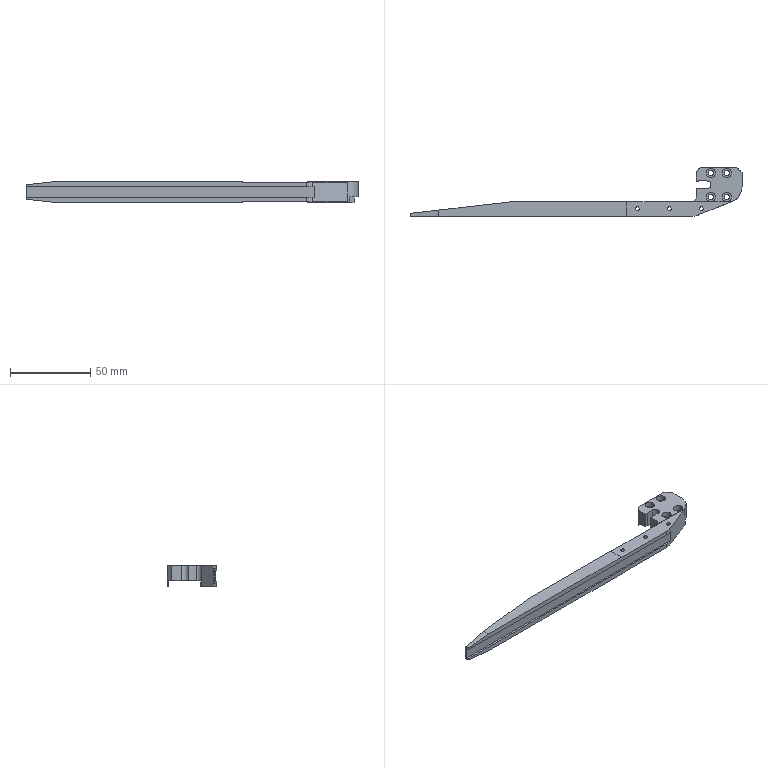Part | 1 solid | 60 faces | box 207.5 x 30.8 x 13 mm | volume 22794 mm3 | plane 41 | cylinder 19 | commonest cylinder face diameters 3.4 x4 5.9 x4 2.5 x3 20 x3 2 x2 1 x1